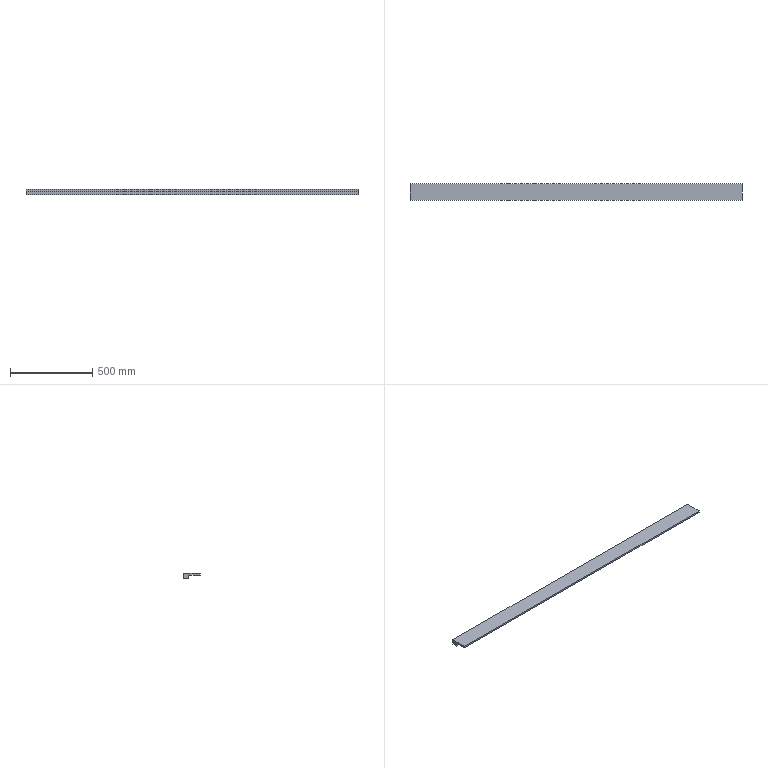Part | STEP file | Linear bearing mounting plate | 1 solid | 8 faces | box 2022 x 100 x 32 mm | volume 3400163 mm3 | plane 8
STEP:
#1=CARTESIAN_POINT('',(0.,0.,0.));
#2=DIRECTION('',(0.,0.,1.));
#3=DIRECTION('',(1.,0.,0.));
#4=AXIS2_PLACEMENT_3D('',#1,#2,#3);
#5=CARTESIAN_POINT('',(1010.75,19.,22.));
#6=VERTEX_POINT('',#5);
#7=CARTESIAN_POINT('',(1010.75,-50.,22.));
#8=VERTEX_POINT('',#7);
#9=CARTESIAN_POINT('',(1010.75,2040.62,22.));
#10=DIRECTION('',(0.,-1.,0.));
#11=VECTOR('',#10,1.);
#12=LINE('',#9,#11);
#13=CARTESIAN_POINT('',(1010.75,50.,32.));
#14=DIRECTION('',(-1.,0.,0.));
#15=DIRECTION('',(0.,0.,1.));
#16=AXIS2_PLACEMENT_3D('',#13,#14,#15);
#17=PLANE('',#16);
#18=CARTESIAN_POINT('',(-10.,1990.62));
#19=DIRECTION('',(0.,-1.));
#20=VECTOR('',#19,1.);
#21=LINE('',#18,#20);
#22=(GEOMETRIC_REPRESENTATION_CONTEXT(2)PARAMETRIC_REPRESENTATION_CONTEXT()REPRESENTATION_CONTEXT('',''));
#23=DEFINITIONAL_REPRESENTATION('',(#21),#22);
#24=PCURVE('',#17,#23);
#25=CARTESIAN_POINT('',(-1010.75,2040.62,22.));
#26=DIRECTION('',(0.,0.,1.));
#27=DIRECTION('',(1.,0.,0.));
#28=AXIS2_PLACEMENT_3D('',#25,#26,#27);
#29=PLANE('',#28);
#30=CARTESIAN_POINT('',(2021.5,0.));
#31=DIRECTION('',(0.,-1.));
#32=VECTOR('',#31,1.);
#33=LINE('',#30,#32);
#34=(GEOMETRIC_REPRESENTATION_CONTEXT(2)PARAMETRIC_REPRESENTATION_CONTEXT()REPRESENTATION_CONTEXT('',''));
#35=DEFINITIONAL_REPRESENTATION('',(#33),#34);
#36=PCURVE('',#29,#35);
#37=SURFACE_CURVE('',#12,(#24,#36),.PCURVE_S1.);
#38=EDGE_CURVE('',#6,#8,#37,.T.);
#39=ORIENTED_EDGE('',*,*,#38,.F.);
#40=CARTESIAN_POINT('',(1010.75,19.,0.));
#41=VERTEX_POINT('',#40);
#42=CARTESIAN_POINT('',(1010.75,19.,0.));
#43=DIRECTION('',(0.,0.,1.));
#44=VECTOR('',#43,1.);
#45=LINE('',#42,#44);
#46=CARTESIAN_POINT('',(-32.,-31.));
#47=DIRECTION('',(1.,0.));
#48=VECTOR('',#47,1.);
#49=LINE('',#46,#48);
#50=(GEOMETRIC_REPRESENTATION_CONTEXT(2)PARAMETRIC_REPRESENTATION_CONTEXT()REPRESENTATION_CONTEXT('',''));
#51=DEFINITIONAL_REPRESENTATION('',(#49),#50);
#52=PCURVE('',#17,#51);
#53=CARTESIAN_POINT('',(1010.75,19.,0.));
#54=DIRECTION('',(0.,1.,0.));
#55=DIRECTION('',(1.,0.,0.));
#56=AXIS2_PLACEMENT_3D('',#53,#54,#55);
#57=PLANE('',#56);
#58=CARTESIAN_POINT('',(0.,0.));
#59=DIRECTION('',(0.,-1.));
#60=VECTOR('',#59,1.);
#61=LINE('',#58,#60);
#62=(GEOMETRIC_REPRESENTATION_CONTEXT(2)PARAMETRIC_REPRESENTATION_CONTEXT()REPRESENTATION_CONTEXT('',''));
#63=DEFINITIONAL_REPRESENTATION('',(#61),#62);
#64=PCURVE('',#57,#63);
#65=SURFACE_CURVE('',#45,(#52,#64),.PCURVE_S1.);
#66=EDGE_CURVE('',#41,#6,#65,.T.);
#67=ORIENTED_EDGE('',*,*,#66,.F.);
#68=CARTESIAN_POINT('',(1010.75,50.,0.));
#69=VERTEX_POINT('',#68);
#70=CARTESIAN_POINT('',(1010.75,50.,0.));
#71=DIRECTION('',(0.,1.,0.));
#72=VECTOR('',#71,1.);
#73=LINE('',#70,#72);
#74=CARTESIAN_POINT('',(-32.,0.));
#75=DIRECTION('',(0.,1.));
#76=VECTOR('',#75,1.);
#77=LINE('',#74,#76);
#78=(GEOMETRIC_REPRESENTATION_CONTEXT(2)PARAMETRIC_REPRESENTATION_CONTEXT()REPRESENTATION_CONTEXT('',''));
#79=DEFINITIONAL_REPRESENTATION('',(#77),#78);
#80=PCURVE('',#17,#79);
#81=CARTESIAN_POINT('',(1010.75,-50.,0.));
#82=DIRECTION('',(0.,0.,1.));
#83=DIRECTION('',(1.,0.,0.));
#84=AXIS2_PLACEMENT_3D('',#81,#82,#83);
#85=PLANE('',#84);
#86=CARTESIAN_POINT('',(0.,100.));
#87=DIRECTION('',(0.,1.));
#88=VECTOR('',#87,1.);
#89=LINE('',#86,#88);
#90=(GEOMETRIC_REPRESENTATION_CONTEXT(2)PARAMETRIC_REPRESENTATION_CONTEXT()REPRESENTATION_CONTEXT('',''));
#91=DEFINITIONAL_REPRESENTATION('',(#89),#90);
#92=PCURVE('',#85,#91);
#93=SURFACE_CURVE('',#73,(#80,#92),.PCURVE_S1.);
#94=EDGE_CURVE('',#41,#69,#93,.T.);
#95=ORIENTED_EDGE('',*,*,#94,.T.);
#96=CARTESIAN_POINT('',(1010.75,50.,32.));
#97=VERTEX_POINT('',#96);
#98=CARTESIAN_POINT('',(1010.75,50.,32.));
#99=DIRECTION('',(0.,0.,-1.));
#100=VECTOR('',#99,1.);
#101=LINE('',#98,#100);
#102=CARTESIAN_POINT('',(0.,0.));
#103=DIRECTION('',(-1.,0.));
#104=VECTOR('',#103,1.);
#105=LINE('',#102,#104);
#106=(GEOMETRIC_REPRESENTATION_CONTEXT(2)PARAMETRIC_REPRESENTATION_CONTEXT()REPRESENTATION_CONTEXT('',''));
#107=DEFINITIONAL_REPRESENTATION('',(#105),#106);
#108=PCURVE('',#17,#107);
#109=CARTESIAN_POINT('',(-1010.75,50.,32.));
#110=DIRECTION('',(0.,-1.,0.));
#111=DIRECTION('',(0.,0.,-1.));
#112=AXIS2_PLACEMENT_3D('',#109,#110,#111);
#113=PLANE('',#112);
#114=CARTESIAN_POINT('',(0.,2021.5));
#115=DIRECTION('',(1.,0.));
#116=VECTOR('',#115,1.);
#117=LINE('',#114,#116);
#118=(GEOMETRIC_REPRESENTATION_CONTEXT(2)PARAMETRIC_REPRESENTATION_CONTEXT()REPRESENTATION_CONTEXT('',''));
#119=DEFINITIONAL_REPRESENTATION('',(#117),#118);
#120=PCURVE('',#113,#119);
#121=SURFACE_CURVE('',#101,(#108,#120),.PCURVE_S1.);
#122=EDGE_CURVE('',#97,#69,#121,.T.);
#123=ORIENTED_EDGE('',*,*,#122,.F.);
#124=CARTESIAN_POINT('',(1010.75,-50.,32.));
#125=VERTEX_POINT('',#124);
#126=CARTESIAN_POINT('',(1010.75,50.,32.));
#127=DIRECTION('',(0.,1.,0.));
#128=VECTOR('',#127,1.);
#129=LINE('',#126,#128);
#130=CARTESIAN_POINT('',(0.,0.));
#131=DIRECTION('',(0.,1.));
#132=VECTOR('',#131,1.);
#133=LINE('',#130,#132);
#134=(GEOMETRIC_REPRESENTATION_CONTEXT(2)PARAMETRIC_REPRESENTATION_CONTEXT()REPRESENTATION_CONTEXT('',''));
#135=DEFINITIONAL_REPRESENTATION('',(#133),#134);
#136=PCURVE('',#17,#135);
#137=CARTESIAN_POINT('',(1010.75,-50.,32.));
#138=DIRECTION('',(0.,0.,1.));
#139=DIRECTION('',(1.,0.,0.));
#140=AXIS2_PLACEMENT_3D('',#137,#138,#139);
#141=PLANE('',#140);
#142=CARTESIAN_POINT('',(0.,100.));
#143=DIRECTION('',(0.,1.));
#144=VECTOR('',#143,1.);
#145=LINE('',#142,#144);
#146=(GEOMETRIC_REPRESENTATION_CONTEXT(2)PARAMETRIC_REPRESENTATION_CONTEXT()REPRESENTATION_CONTEXT('',''));
#147=DEFINITIONAL_REPRESENTATION('',(#145),#146);
#148=PCURVE('',#141,#147);
#149=SURFACE_CURVE('',#129,(#136,#148),.PCURVE_S1.);
#150=EDGE_CURVE('',#125,#97,#149,.T.);
#151=ORIENTED_EDGE('',*,*,#150,.F.);
#152=CARTESIAN_POINT('',(1010.75,-50.,32.));
#153=DIRECTION('',(0.,0.,-1.));
#154=VECTOR('',#153,1.);
#155=LINE('',#152,#154);
#156=CARTESIAN_POINT('',(0.,-100.));
#157=DIRECTION('',(-1.,0.));
#158=VECTOR('',#157,1.);
#159=LINE('',#156,#158);
#160=(GEOMETRIC_REPRESENTATION_CONTEXT(2)PARAMETRIC_REPRESENTATION_CONTEXT()REPRESENTATION_CONTEXT('',''));
#161=DEFINITIONAL_REPRESENTATION('',(#159),#160);
#162=PCURVE('',#17,#161);
#163=CARTESIAN_POINT('',(-1010.75,-50.,32.));
#164=DIRECTION('',(0.,1.,0.));
#165=DIRECTION('',(0.,0.,1.));
#166=AXIS2_PLACEMENT_3D('',#163,#164,#165);
#167=PLANE('',#166);
#168=CARTESIAN_POINT('',(0.,2021.5));
#169=DIRECTION('',(-1.,0.));
#170=VECTOR('',#169,1.);
#171=LINE('',#168,#170);
#172=(GEOMETRIC_REPRESENTATION_CONTEXT(2)PARAMETRIC_REPRESENTATION_CONTEXT()REPRESENTATION_CONTEXT('',''));
#173=DEFINITIONAL_REPRESENTATION('',(#171),#172);
#174=PCURVE('',#167,#173);
#175=SURFACE_CURVE('',#155,(#162,#174),.PCURVE_S1.);
#176=EDGE_CURVE('',#125,#8,#175,.T.);
#177=ORIENTED_EDGE('',*,*,#176,.T.);
#178=EDGE_LOOP('',(#39,#67,#95,#123,#151,#177));
#179=FACE_BOUND('',#178,.T.);
#180=ADVANCED_FACE('',(#179),#17,.F.);
#181=CARTESIAN_POINT('',(-1010.75,50.,0.));
#182=VERTEX_POINT('',#181);
#183=CARTESIAN_POINT('',(-1010.75,50.,0.));
#184=DIRECTION('',(-1.,0.,0.));
#185=VECTOR('',#184,1.);
#186=LINE('',#183,#185);
#187=CARTESIAN_POINT('',(32.,0.));
#188=DIRECTION('',(0.,-1.));
#189=VECTOR('',#188,1.);
#190=LINE('',#187,#189);
#191=(GEOMETRIC_REPRESENTATION_CONTEXT(2)PARAMETRIC_REPRESENTATION_CONTEXT()REPRESENTATION_CONTEXT('',''));
#192=DEFINITIONAL_REPRESENTATION('',(#190),#191);
#193=PCURVE('',#113,#192);
#194=CARTESIAN_POINT('',(-2021.5,100.));
#195=DIRECTION('',(-1.,0.));
#196=VECTOR('',#195,1.);
#197=LINE('',#194,#196);
#198=(GEOMETRIC_REPRESENTATION_CONTEXT(2)PARAMETRIC_REPRESENTATION_CONTEXT()REPRESENTATION_CONTEXT('',''));
#199=DEFINITIONAL_REPRESENTATION('',(#197),#198);
#200=PCURVE('',#85,#199);
#201=SURFACE_CURVE('',#186,(#193,#200),.PCURVE_S1.);
#202=EDGE_CURVE('',#69,#182,#201,.T.);
#203=ORIENTED_EDGE('',*,*,#202,.T.);
#204=CARTESIAN_POINT('',(-1010.75,50.,32.));
#205=VERTEX_POINT('',#204);
#206=CARTESIAN_POINT('',(-1010.75,50.,32.));
#207=DIRECTION('',(0.,0.,-1.));
#208=VECTOR('',#207,1.);
#209=LINE('',#206,#208);
#210=CARTESIAN_POINT('',(0.,0.));
#211=DIRECTION('',(1.,0.));
#212=VECTOR('',#211,1.);
#213=LINE('',#210,#212);
#214=(GEOMETRIC_REPRESENTATION_CONTEXT(2)PARAMETRIC_REPRESENTATION_CONTEXT()REPRESENTATION_CONTEXT('',''));
#215=DEFINITIONAL_REPRESENTATION('',(#213),#214);
#216=PCURVE('',#113,#215);
#217=CARTESIAN_POINT('',(-1010.75,50.,32.));
#218=DIRECTION('',(1.,0.,0.));
#219=DIRECTION('',(0.,0.,-1.));
#220=AXIS2_PLACEMENT_3D('',#217,#218,#219);
#221=PLANE('',#220);
#222=CARTESIAN_POINT('',(0.,0.));
#223=DIRECTION('',(1.,0.));
#224=VECTOR('',#223,1.);
#225=LINE('',#222,#224);
#226=(GEOMETRIC_REPRESENTATION_CONTEXT(2)PARAMETRIC_REPRESENTATION_CONTEXT()REPRESENTATION_CONTEXT('',''));
#227=DEFINITIONAL_REPRESENTATION('',(#225),#226);
#228=PCURVE('',#221,#227);
#229=SURFACE_CURVE('',#209,(#216,#228),.PCURVE_S1.);
#230=EDGE_CURVE('',#205,#182,#229,.T.);
#231=ORIENTED_EDGE('',*,*,#230,.F.);
#232=CARTESIAN_POINT('',(-1010.75,50.,32.));
#233=DIRECTION('',(-1.,0.,0.));
#234=VECTOR('',#233,1.);
#235=LINE('',#232,#234);
#236=CARTESIAN_POINT('',(0.,0.));
#237=DIRECTION('',(0.,-1.));
#238=VECTOR('',#237,1.);
#239=LINE('',#236,#238);
#240=(GEOMETRIC_REPRESENTATION_CONTEXT(2)PARAMETRIC_REPRESENTATION_CONTEXT()REPRESENTATION_CONTEXT('',''));
#241=DEFINITIONAL_REPRESENTATION('',(#239),#240);
#242=PCURVE('',#113,#241);
#243=CARTESIAN_POINT('',(-2021.5,100.));
#244=DIRECTION('',(-1.,0.));
#245=VECTOR('',#244,1.);
#246=LINE('',#243,#245);
#247=(GEOMETRIC_REPRESENTATION_CONTEXT(2)PARAMETRIC_REPRESENTATION_CONTEXT()REPRESENTATION_CONTEXT('',''));
#248=DEFINITIONAL_REPRESENTATION('',(#246),#247);
#249=PCURVE('',#141,#248);
#250=SURFACE_CURVE('',#235,(#242,#249),.PCURVE_S1.);
#251=EDGE_CURVE('',#97,#205,#250,.T.);
#252=ORIENTED_EDGE('',*,*,#251,.F.);
#253=ORIENTED_EDGE('',*,*,#122,.T.);
#254=EDGE_LOOP('',(#203,#231,#252,#253));
#255=FACE_BOUND('',#254,.T.);
#256=ADVANCED_FACE('',(#255),#113,.F.);
#257=CARTESIAN_POINT('',(-1010.75,19.,0.));
#258=VERTEX_POINT('',#257);
#259=CARTESIAN_POINT('',(-1010.75,50.,0.));
#260=DIRECTION('',(0.,-1.,0.));
#261=VECTOR('',#260,1.);
#262=LINE('',#259,#261);
#263=CARTESIAN_POINT('',(32.,0.));
#264=DIRECTION('',(0.,-1.));
#265=VECTOR('',#264,1.);
#266=LINE('',#263,#265);
#267=(GEOMETRIC_REPRESENTATION_CONTEXT(2)PARAMETRIC_REPRESENTATION_CONTEXT()REPRESENTATION_CONTEXT('',''));
#268=DEFINITIONAL_REPRESENTATION('',(#266),#267);
#269=PCURVE('',#221,#268);
#270=CARTESIAN_POINT('',(-2021.5,100.));
#271=DIRECTION('',(0.,-1.));
#272=VECTOR('',#271,1.);
#273=LINE('',#270,#272);
#274=(GEOMETRIC_REPRESENTATION_CONTEXT(2)PARAMETRIC_REPRESENTATION_CONTEXT()REPRESENTATION_CONTEXT('',''));
#275=DEFINITIONAL_REPRESENTATION('',(#273),#274);
#276=PCURVE('',#85,#275);
#277=SURFACE_CURVE('',#262,(#269,#276),.PCURVE_S1.);
#278=EDGE_CURVE('',#182,#258,#277,.T.);
#279=ORIENTED_EDGE('',*,*,#278,.T.);
#280=CARTESIAN_POINT('',(-1010.75,19.,22.));
#281=VERTEX_POINT('',#280);
#282=CARTESIAN_POINT('',(-1010.75,19.,0.));
#283=DIRECTION('',(0.,0.,-1.));
#284=VECTOR('',#283,1.);
#285=LINE('',#282,#284);
#286=CARTESIAN_POINT('',(32.,-31.));
#287=DIRECTION('',(1.,0.));
#288=VECTOR('',#287,1.);
#289=LINE('',#286,#288);
#290=(GEOMETRIC_REPRESENTATION_CONTEXT(2)PARAMETRIC_REPRESENTATION_CONTEXT()REPRESENTATION_CONTEXT('',''));
#291=DEFINITIONAL_REPRESENTATION('',(#289),#290);
#292=PCURVE('',#221,#291);
#293=CARTESIAN_POINT('',(-2021.5,0.));
#294=DIRECTION('',(0.,1.));
#295=VECTOR('',#294,1.);
#296=LINE('',#293,#295);
#297=(GEOMETRIC_REPRESENTATION_CONTEXT(2)PARAMETRIC_REPRESENTATION_CONTEXT()REPRESENTATION_CONTEXT('',''));
#298=DEFINITIONAL_REPRESENTATION('',(#296),#297);
#299=PCURVE('',#57,#298);
#300=SURFACE_CURVE('',#285,(#292,#299),.PCURVE_S1.);
#301=EDGE_CURVE('',#281,#258,#300,.T.);
#302=ORIENTED_EDGE('',*,*,#301,.F.);
#303=CARTESIAN_POINT('',(-1010.75,-50.,22.));
#304=VERTEX_POINT('',#303);
#305=CARTESIAN_POINT('',(-1010.75,2040.62,22.));
#306=DIRECTION('',(0.,-1.,0.));
#307=VECTOR('',#306,1.);
#308=LINE('',#305,#307);
#309=CARTESIAN_POINT('',(10.,1990.62));
#310=DIRECTION('',(0.,-1.));
#311=VECTOR('',#310,1.);
#312=LINE('',#309,#311);
#313=(GEOMETRIC_REPRESENTATION_CONTEXT(2)PARAMETRIC_REPRESENTATION_CONTEXT()REPRESENTATION_CONTEXT('',''));
#314=DEFINITIONAL_REPRESENTATION('',(#312),#313);
#315=PCURVE('',#221,#314);
#316=CARTESIAN_POINT('',(0.,0.));
#317=DIRECTION('',(0.,-1.));
#318=VECTOR('',#317,1.);
#319=LINE('',#316,#318);
#320=(GEOMETRIC_REPRESENTATION_CONTEXT(2)PARAMETRIC_REPRESENTATION_CONTEXT()REPRESENTATION_CONTEXT('',''));
#321=DEFINITIONAL_REPRESENTATION('',(#319),#320);
#322=PCURVE('',#29,#321);
#323=SURFACE_CURVE('',#308,(#315,#322),.PCURVE_S1.);
#324=EDGE_CURVE('',#281,#304,#323,.T.);
#325=ORIENTED_EDGE('',*,*,#324,.T.);
#326=CARTESIAN_POINT('',(-1010.75,-50.,32.));
#327=VERTEX_POINT('',#326);
#328=CARTESIAN_POINT('',(-1010.75,-50.,32.));
#329=DIRECTION('',(0.,0.,-1.));
#330=VECTOR('',#329,1.);
#331=LINE('',#328,#330);
#332=CARTESIAN_POINT('',(0.,-100.));
#333=DIRECTION('',(1.,0.));
#334=VECTOR('',#333,1.);
#335=LINE('',#332,#334);
#336=(GEOMETRIC_REPRESENTATION_CONTEXT(2)PARAMETRIC_REPRESENTATION_CONTEXT()REPRESENTATION_CONTEXT('',''));
#337=DEFINITIONAL_REPRESENTATION('',(#335),#336);
#338=PCURVE('',#221,#337);
#339=CARTESIAN_POINT('',(0.,0.));
#340=DIRECTION('',(-1.,0.));
#341=VECTOR('',#340,1.);
#342=LINE('',#339,#341);
#343=(GEOMETRIC_REPRESENTATION_CONTEXT(2)PARAMETRIC_REPRESENTATION_CONTEXT()REPRESENTATION_CONTEXT('',''));
#344=DEFINITIONAL_REPRESENTATION('',(#342),#343);
#345=PCURVE('',#167,#344);
#346=SURFACE_CURVE('',#331,(#338,#345),.PCURVE_S1.);
#347=EDGE_CURVE('',#327,#304,#346,.T.);
#348=ORIENTED_EDGE('',*,*,#347,.F.);
#349=CARTESIAN_POINT('',(-1010.75,50.,32.));
#350=DIRECTION('',(0.,-1.,0.));
#351=VECTOR('',#350,1.);
#352=LINE('',#349,#351);
#353=CARTESIAN_POINT('',(0.,0.));
#354=DIRECTION('',(0.,-1.));
#355=VECTOR('',#354,1.);
#356=LINE('',#353,#355);
#357=(GEOMETRIC_REPRESENTATION_CONTEXT(2)PARAMETRIC_REPRESENTATION_CONTEXT()REPRESENTATION_CONTEXT('',''));
#358=DEFINITIONAL_REPRESENTATION('',(#356),#357);
#359=PCURVE('',#221,#358);
#360=CARTESIAN_POINT('',(-2021.5,100.));
#361=DIRECTION('',(0.,-1.));
#362=VECTOR('',#361,1.);
#363=LINE('',#360,#362);
#364=(GEOMETRIC_REPRESENTATION_CONTEXT(2)PARAMETRIC_REPRESENTATION_CONTEXT()REPRESENTATION_CONTEXT('',''));
#365=DEFINITIONAL_REPRESENTATION('',(#363),#364);
#366=PCURVE('',#141,#365);
#367=SURFACE_CURVE('',#352,(#359,#366),.PCURVE_S1.);
#368=EDGE_CURVE('',#205,#327,#367,.T.);
#369=ORIENTED_EDGE('',*,*,#368,.F.);
#370=ORIENTED_EDGE('',*,*,#230,.T.);
#371=EDGE_LOOP('',(#279,#302,#325,#348,#369,#370));
#372=FACE_BOUND('',#371,.T.);
#373=ADVANCED_FACE('',(#372),#221,.F.);
#374=ORIENTED_EDGE('',*,*,#347,.T.);
#375=CARTESIAN_POINT('',(-1010.75,-50.,22.));
#376=DIRECTION('',(-1.,0.,0.));
#377=VECTOR('',#376,1.);
#378=LINE('',#375,#377);
#379=CARTESIAN_POINT('',(-10.,0.));
#380=DIRECTION('',(0.,-1.));
#381=VECTOR('',#380,1.);
#382=LINE('',#379,#381);
#383=(GEOMETRIC_REPRESENTATION_CONTEXT(2)PARAMETRIC_REPRESENTATION_CONTEXT()REPRESENTATION_CONTEXT('',''));
#384=DEFINITIONAL_REPRESENTATION('',(#382),#383);
#385=PCURVE('',#167,#384);
#386=CARTESIAN_POINT('',(0.,-2090.62));
#387=DIRECTION('',(-1.,0.));
#388=VECTOR('',#387,1.);
#389=LINE('',#386,#388);
#390=(GEOMETRIC_REPRESENTATION_CONTEXT(2)PARAMETRIC_REPRESENTATION_CONTEXT()REPRESENTATION_CONTEXT('',''));
#391=DEFINITIONAL_REPRESENTATION('',(#389),#390);
#392=PCURVE('',#29,#391);
#393=SURFACE_CURVE('',#378,(#385,#392),.PCURVE_S1.);
#394=EDGE_CURVE('',#8,#304,#393,.T.);
#395=ORIENTED_EDGE('',*,*,#394,.F.);
#396=ORIENTED_EDGE('',*,*,#176,.F.);
#397=CARTESIAN_POINT('',(-1010.75,-50.,32.));
#398=DIRECTION('',(1.,0.,0.));
#399=VECTOR('',#398,1.);
#400=LINE('',#397,#399);
#401=CARTESIAN_POINT('',(0.,0.));
#402=DIRECTION('',(0.,1.));
#403=VECTOR('',#402,1.);
#404=LINE('',#401,#403);
#405=(GEOMETRIC_REPRESENTATION_CONTEXT(2)PARAMETRIC_REPRESENTATION_CONTEXT()REPRESENTATION_CONTEXT('',''));
#406=DEFINITIONAL_REPRESENTATION('',(#404),#405);
#407=PCURVE('',#167,#406);
#408=CARTESIAN_POINT('',(-2021.5,0.));
#409=DIRECTION('',(1.,0.));
#410=VECTOR('',#409,1.);
#411=LINE('',#408,#410);
#412=(GEOMETRIC_REPRESENTATION_CONTEXT(2)PARAMETRIC_REPRESENTATION_CONTEXT()REPRESENTATION_CONTEXT('',''));
#413=DEFINITIONAL_REPRESENTATION('',(#411),#412);
#414=PCURVE('',#141,#413);
#415=SURFACE_CURVE('',#400,(#407,#414),.PCURVE_S1.);
#416=EDGE_CURVE('',#327,#125,#415,.T.);
#417=ORIENTED_EDGE('',*,*,#416,.F.);
#418=EDGE_LOOP('',(#374,#395,#396,#417));
#419=FACE_BOUND('',#418,.T.);
#420=ADVANCED_FACE('',(#419),#167,.F.);
#421=ORIENTED_EDGE('',*,*,#150,.T.);
#422=ORIENTED_EDGE('',*,*,#251,.T.);
#423=ORIENTED_EDGE('',*,*,#368,.T.);
#424=ORIENTED_EDGE('',*,*,#416,.T.);
#425=EDGE_LOOP('',(#421,#422,#423,#424));
#426=FACE_BOUND('',#425,.T.);
#427=ADVANCED_FACE('',(#426),#141,.T.);
#428=ORIENTED_EDGE('',*,*,#94,.F.);
#429=CARTESIAN_POINT('',(-1010.75,19.,0.));
#430=DIRECTION('',(1.,0.,0.));
#431=VECTOR('',#430,1.);
#432=LINE('',#429,#431);
#433=CARTESIAN_POINT('',(-2021.5,69.));
#434=DIRECTION('',(1.,0.));
#435=VECTOR('',#434,1.);
#436=LINE('',#433,#435);
#437=(GEOMETRIC_REPRESENTATION_CONTEXT(2)PARAMETRIC_REPRESENTATION_CONTEXT()REPRESENTATION_CONTEXT('',''));
#438=DEFINITIONAL_REPRESENTATION('',(#436),#437);
#439=PCURVE('',#85,#438);
#440=CARTESIAN_POINT('',(-2021.5,0.));
#441=DIRECTION('',(1.,0.));
#442=VECTOR('',#441,1.);
#443=LINE('',#440,#442);
#444=(GEOMETRIC_REPRESENTATION_CONTEXT(2)PARAMETRIC_REPRESENTATION_CONTEXT()REPRESENTATION_CONTEXT('',''));
#445=DEFINITIONAL_REPRESENTATION('',(#443),#444);
#446=PCURVE('',#57,#445);
#447=SURFACE_CURVE('',#432,(#439,#446),.PCURVE_S1.);
#448=EDGE_CURVE('',#258,#41,#447,.T.);
#449=ORIENTED_EDGE('',*,*,#448,.F.);
#450=ORIENTED_EDGE('',*,*,#278,.F.);
#451=ORIENTED_EDGE('',*,*,#202,.F.);
#452=EDGE_LOOP('',(#428,#449,#450,#451));
#453=FACE_BOUND('',#452,.T.);
#454=ADVANCED_FACE('',(#453),#85,.F.);
#455=ORIENTED_EDGE('',*,*,#301,.T.);
#456=ORIENTED_EDGE('',*,*,#448,.T.);
#457=ORIENTED_EDGE('',*,*,#66,.T.);
#458=CARTESIAN_POINT('',(-1010.75,19.,22.));
#459=DIRECTION('',(-1.,0.,0.));
#460=VECTOR('',#459,1.);
#461=LINE('',#458,#460);
#462=CARTESIAN_POINT('',(-2021.5,-22.));
#463=DIRECTION('',(-1.,0.));
#464=VECTOR('',#463,1.);
#465=LINE('',#462,#464);
#466=(GEOMETRIC_REPRESENTATION_CONTEXT(2)PARAMETRIC_REPRESENTATION_CONTEXT()REPRESENTATION_CONTEXT('',''));
#467=DEFINITIONAL_REPRESENTATION('',(#465),#466);
#468=PCURVE('',#57,#467);
#469=CARTESIAN_POINT('',(0.,-2021.62));
#470=DIRECTION('',(-1.,0.));
#471=VECTOR('',#470,1.);
#472=LINE('',#469,#471);
#473=(GEOMETRIC_REPRESENTATION_CONTEXT(2)PARAMETRIC_REPRESENTATION_CONTEXT()REPRESENTATION_CONTEXT('',''));
#474=DEFINITIONAL_REPRESENTATION('',(#472),#473);
#475=PCURVE('',#29,#474);
#476=SURFACE_CURVE('',#461,(#468,#475),.PCURVE_S1.);
#477=EDGE_CURVE('',#6,#281,#476,.T.);
#478=ORIENTED_EDGE('',*,*,#477,.T.);
#479=EDGE_LOOP('',(#455,#456,#457,#478));
#480=FACE_BOUND('',#479,.T.);
#481=ADVANCED_FACE('',(#480),#57,.F.);
#482=ORIENTED_EDGE('',*,*,#38,.T.);
#483=ORIENTED_EDGE('',*,*,#394,.T.);
#484=ORIENTED_EDGE('',*,*,#324,.F.);
#485=ORIENTED_EDGE('',*,*,#477,.F.);
#486=EDGE_LOOP('',(#482,#483,#484,#485));
#487=FACE_BOUND('',#486,.T.);
#488=ADVANCED_FACE('',(#487),#29,.F.);
#489=CLOSED_SHELL('',(#180,#256,#373,#420,#427,#454,#481,#488));
#490=MANIFOLD_SOLID_BREP('',#489);
#491=(LENGTH_UNIT()NAMED_UNIT(*)SI_UNIT(.MILLI.,.METRE.));
#492=UNCERTAINTY_MEASURE_WITH_UNIT(LENGTH_MEASURE(0.0000001),#491,'','');
#493=(NAMED_UNIT(*)PLANE_ANGLE_UNIT()SI_UNIT($,.RADIAN.));
#494=(NAMED_UNIT(*)SI_UNIT($,.STERADIAN.)SOLID_ANGLE_UNIT());
#495=(GEOMETRIC_REPRESENTATION_CONTEXT(3)GLOBAL_UNCERTAINTY_ASSIGNED_CONTEXT((#492))GLOBAL_UNIT_ASSIGNED_CONTEXT((#491,#493,#494))REPRESENTATION_CONTEXT('',''));
#496=ADVANCED_BREP_SHAPE_REPRESENTATION('',(#4,#490),#495);